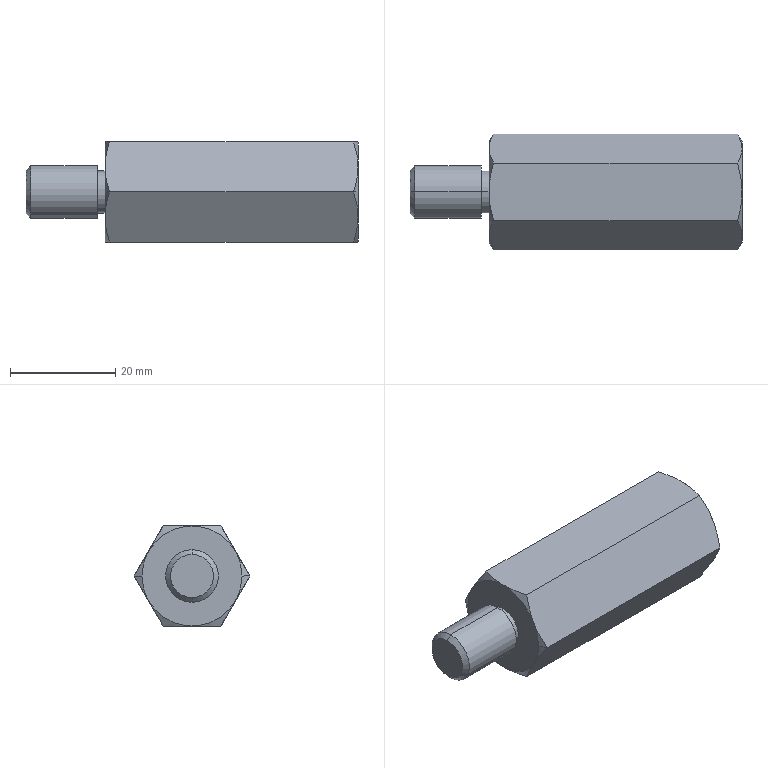Part | STEP file | 0228_004_SLSBG19-48-M10-N8 | 1 solid | 26 faces | box 63 x 21.939 x 19 mm | volume 15277 mm3 | cone 10 | plane 10 | cylinder 6 | commonest cylinder face diameters 6.8 x2 8 x2 10 x2